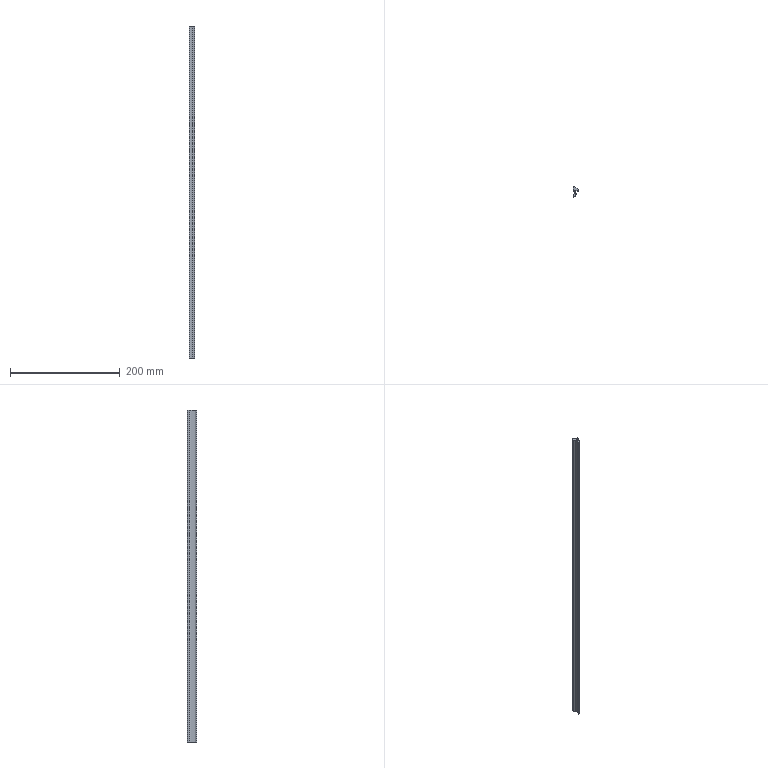Part | SolidWorks | features BaseBody 1, MoveFace 1 | 1 solid | 20 faces | box 10.8 x 17.5 x 606 mm | volume 47753 mm3 | cylinder 11 | plane 9 | commonest cylinder face diameters 1.6 x2 14 x2 0.4 x1 0.6 x1 0.8 x1 2.6 x1
STEP:
#1=CARTESIAN_POINT('',(-3.236,-11.055,506.));
#2=VERTEX_POINT('',#1);
#3=CARTESIAN_POINT('',(-4.3,-10.3,506.));
#4=VERTEX_POINT('',#3);
#5=CARTESIAN_POINT('',(-3.5,-10.3,506.));
#6=DIRECTION('',(0.,0.,-1.));
#7=DIRECTION('',(1.,0.,0.));
#8=AXIS2_PLACEMENT_3D('',#5,#6,#7);
#9=CIRCLE('',#8,0.8);
#10=EDGE_CURVE('',#2,#4,#9,.T.);
#11=ORIENTED_EDGE('',*,*,#10,.T.);
#12=CARTESIAN_POINT('',(-4.3,-10.3,-100.));
#13=VERTEX_POINT('',#12);
#14=CARTESIAN_POINT('',(-4.3,-10.3,-100.));
#15=DIRECTION('',(0.,0.,-1.));
#16=VECTOR('',#15,1000.);
#17=LINE('',#14,#16);
#18=EDGE_CURVE('',#4,#13,#17,.T.);
#19=ORIENTED_EDGE('',*,*,#18,.T.);
#20=CARTESIAN_POINT('',(-3.236,-11.055,-100.));
#21=VERTEX_POINT('',#20);
#22=CARTESIAN_POINT('',(-3.5,-10.3,-100.));
#23=DIRECTION('',(0.,0.,1.));
#24=DIRECTION('',(-1.,0.,0.));
#25=AXIS2_PLACEMENT_3D('',#22,#23,#24);
#26=CIRCLE('',#25,0.8);
#27=EDGE_CURVE('',#13,#21,#26,.T.);
#28=ORIENTED_EDGE('',*,*,#27,.T.);
#29=CARTESIAN_POINT('',(-3.236,-11.055,-100.));
#30=DIRECTION('',(0.,0.,-1.));
#31=VECTOR('',#30,1000.);
#32=LINE('',#29,#31);
#33=EDGE_CURVE('',#2,#21,#32,.T.);
#34=ORIENTED_EDGE('',*,*,#33,.F.);
#35=EDGE_LOOP('',(#11,#19,#28,#34));
#36=FACE_OUTER_BOUND('',#35,.T.);
#37=CARTESIAN_POINT('',(-3.5,-10.3,-100.));
#38=DIRECTION('',(0.,0.,-1.));
#39=DIRECTION('',(-1.,0.,0.));
#40=AXIS2_PLACEMENT_3D('',#37,#38,#39);
#41=CYLINDRICAL_SURFACE('',#40,0.8);
#42=ADVANCED_FACE('',(#36),#41,.T.);
#43=CARTESIAN_POINT('',(1.184,-6.397,-100.));
#44=VERTEX_POINT('',#43);
#45=CARTESIAN_POINT('',(-5.702,-4.29,-100.));
#46=DIRECTION('',(0.,0.,1.));
#47=DIRECTION('',(-1.,0.,0.));
#48=AXIS2_PLACEMENT_3D('',#45,#46,#47);
#49=CIRCLE('',#48,7.201);
#50=EDGE_CURVE('',#21,#44,#49,.T.);
#51=ORIENTED_EDGE('',*,*,#50,.T.);
#52=CARTESIAN_POINT('',(1.184,-6.397,506.));
#53=VERTEX_POINT('',#52);
#54=CARTESIAN_POINT('',(1.184,-6.397,-100.));
#55=DIRECTION('',(0.,0.,1.));
#56=VECTOR('',#55,1000.);
#57=LINE('',#54,#56);
#58=EDGE_CURVE('',#44,#53,#57,.T.);
#59=ORIENTED_EDGE('',*,*,#58,.T.);
#60=CARTESIAN_POINT('',(-5.702,-4.29,506.));
#61=DIRECTION('',(0.,0.,-1.));
#62=DIRECTION('',(1.,0.,0.));
#63=AXIS2_PLACEMENT_3D('',#60,#61,#62);
#64=CIRCLE('',#63,7.201);
#65=EDGE_CURVE('',#53,#2,#64,.T.);
#66=ORIENTED_EDGE('',*,*,#65,.T.);
#67=ORIENTED_EDGE('',*,*,#33,.T.);
#68=EDGE_LOOP('',(#51,#59,#66,#67));
#69=FACE_OUTER_BOUND('',#68,.T.);
#70=CARTESIAN_POINT('',(-5.702,-4.29,-100.));
#71=DIRECTION('',(0.,0.,-1.));
#72=DIRECTION('',(-1.,0.,0.));
#73=AXIS2_PLACEMENT_3D('',#70,#71,#72);
#74=CYLINDRICAL_SURFACE('',#73,7.201);
#75=ADVANCED_FACE('',(#69),#74,.T.);
#76=CARTESIAN_POINT('',(0.9,-6.,-100.));
#77=VERTEX_POINT('',#76);
#78=CARTESIAN_POINT('',(0.9,-6.3,-100.));
#79=DIRECTION('',(0.,0.,1.));
#80=DIRECTION('',(-1.,0.,0.));
#81=AXIS2_PLACEMENT_3D('',#78,#79,#80);
#82=CIRCLE('',#81,0.3);
#83=EDGE_CURVE('',#44,#77,#82,.T.);
#84=ORIENTED_EDGE('',*,*,#83,.T.);
#85=CARTESIAN_POINT('',(0.9,-6.,506.));
#86=VERTEX_POINT('',#85);
#87=CARTESIAN_POINT('',(0.9,-6.,-100.));
#88=DIRECTION('',(0.,0.,1.));
#89=VECTOR('',#88,1000.);
#90=LINE('',#87,#89);
#91=EDGE_CURVE('',#77,#86,#90,.T.);
#92=ORIENTED_EDGE('',*,*,#91,.T.);
#93=CARTESIAN_POINT('',(0.9,-6.3,506.));
#94=DIRECTION('',(0.,0.,-1.));
#95=DIRECTION('',(1.,0.,0.));
#96=AXIS2_PLACEMENT_3D('',#93,#94,#95);
#97=CIRCLE('',#96,0.3);
#98=EDGE_CURVE('',#86,#53,#97,.T.);
#99=ORIENTED_EDGE('',*,*,#98,.T.);
#100=ORIENTED_EDGE('',*,*,#58,.F.);
#101=EDGE_LOOP('',(#84,#92,#99,#100));
#102=FACE_OUTER_BOUND('',#101,.T.);
#103=CARTESIAN_POINT('',(0.9,-6.3,-100.));
#104=DIRECTION('',(0.,0.,-1.));
#105=DIRECTION('',(-1.,0.,0.));
#106=AXIS2_PLACEMENT_3D('',#103,#104,#105);
#107=CYLINDRICAL_SURFACE('',#106,0.3);
#108=ADVANCED_FACE('',(#102),#107,.T.);
#109=CARTESIAN_POINT('',(-2.5,-0.5,-100.));
#110=VERTEX_POINT('',#109);
#111=CARTESIAN_POINT('',(-2.5,-6.153,-100.));
#112=VERTEX_POINT('',#111);
#113=CARTESIAN_POINT('',(-2.5,-6.397,-100.));
#114=DIRECTION('',(0.,-1.,0.));
#115=VECTOR('',#114,1000.);
#116=LINE('',#113,#115);
#117=EDGE_CURVE('',#110,#112,#116,.T.);
#118=ORIENTED_EDGE('',*,*,#117,.F.);
#119=CARTESIAN_POINT('',(-4.2,1.695,-100.));
#120=VERTEX_POINT('',#119);
#121=CARTESIAN_POINT('',(-1.701,1.875,-100.));
#122=DIRECTION('',(0.,0.,1.));
#123=DIRECTION('',(-1.,0.,0.));
#124=AXIS2_PLACEMENT_3D('',#121,#122,#123);
#125=CIRCLE('',#124,2.506);
#126=EDGE_CURVE('',#120,#110,#125,.T.);
#127=ORIENTED_EDGE('',*,*,#126,.F.);
#128=CARTESIAN_POINT('',(-4.2,5.1,-100.));
#129=VERTEX_POINT('',#128);
#130=CARTESIAN_POINT('',(-4.2,-6.397,-100.));
#131=DIRECTION('',(0.,-1.,0.));
#132=VECTOR('',#131,1000.);
#133=LINE('',#130,#132);
#134=EDGE_CURVE('',#129,#120,#133,.T.);
#135=ORIENTED_EDGE('',*,*,#134,.F.);
#136=CARTESIAN_POINT('',(-2.892,6.4,-100.));
#137=VERTEX_POINT('',#136);
#138=CARTESIAN_POINT('',(-2.9,5.1,-100.));
#139=DIRECTION('',(0.,0.,1.));
#140=DIRECTION('',(-1.,0.,0.));
#141=AXIS2_PLACEMENT_3D('',#138,#139,#140);
#142=CIRCLE('',#141,1.3);
#143=EDGE_CURVE('',#137,#129,#142,.T.);
#144=ORIENTED_EDGE('',*,*,#143,.F.);
#145=CARTESIAN_POINT('',(0.5,5.5,-100.));
#146=VERTEX_POINT('',#145);
#147=CARTESIAN_POINT('',(-2.934,-0.5999,-100.));
#148=DIRECTION('',(0.,0.,1.));
#149=DIRECTION('',(-1.,0.,0.));
#150=AXIS2_PLACEMENT_3D('',#147,#148,#149);
#151=CIRCLE('',#150,7.);
#152=EDGE_CURVE('',#146,#137,#151,.T.);
#153=ORIENTED_EDGE('',*,*,#152,.F.);
#154=CARTESIAN_POINT('',(5.5,1.7,-100.));
#155=VERTEX_POINT('',#154);
#156=CARTESIAN_POINT('',(5.5,1.7,-100.));
#157=DIRECTION('',(-0.7962,0.6051,0.));
#158=VECTOR('',#157,1000.);
#159=LINE('',#156,#158);
#160=EDGE_CURVE('',#155,#146,#159,.T.);
#161=ORIENTED_EDGE('',*,*,#160,.F.);
#162=CARTESIAN_POINT('',(6.458,-0.2215,-100.));
#163=VERTEX_POINT('',#162);
#164=CARTESIAN_POINT('',(6.458,-0.2215,-100.));
#165=DIRECTION('',(-0.4462,0.8949,0.));
#166=VECTOR('',#165,1000.);
#167=LINE('',#164,#166);
#168=EDGE_CURVE('',#163,#155,#167,.T.);
#169=ORIENTED_EDGE('',*,*,#168,.F.);
#170=CARTESIAN_POINT('',(5.895,-0.7433,-100.));
#171=VERTEX_POINT('',#170);
#172=CARTESIAN_POINT('',(6.1,-0.4,-100.));
#173=DIRECTION('',(0.,0.,1.));
#174=DIRECTION('',(-1.,0.,0.));
#175=AXIS2_PLACEMENT_3D('',#172,#173,#174);
#176=CIRCLE('',#175,0.4);
#177=EDGE_CURVE('',#171,#163,#176,.T.);
#178=ORIENTED_EDGE('',*,*,#177,.F.);
#179=CARTESIAN_POINT('',(3.,0.,-100.));
#180=VERTEX_POINT('',#179);
#181=CARTESIAN_POINT('',(2.746,-6.995,-100.));
#182=DIRECTION('',(0.,0.,-1.));
#183=DIRECTION('',(-1.,0.,0.));
#184=AXIS2_PLACEMENT_3D('',#181,#182,#183);
#185=CIRCLE('',#184,7.);
#186=EDGE_CURVE('',#180,#171,#185,.T.);
#187=ORIENTED_EDGE('',*,*,#186,.F.);
#188=CARTESIAN_POINT('',(0.,0.,-100.));
#189=VERTEX_POINT('',#188);
#190=CARTESIAN_POINT('',(-6.814,0.,-100.));
#191=DIRECTION('',(1.,0.,0.));
#192=VECTOR('',#191,1000.);
#193=LINE('',#190,#192);
#194=EDGE_CURVE('',#189,#180,#193,.T.);
#195=ORIENTED_EDGE('',*,*,#194,.F.);
#196=CARTESIAN_POINT('',(0.,-5.8,-100.));
#197=VERTEX_POINT('',#196);
#198=CARTESIAN_POINT('',(0.,-6.397,-100.));
#199=DIRECTION('',(0.,1.,0.));
#200=VECTOR('',#199,1000.);
#201=LINE('',#198,#200);
#202=EDGE_CURVE('',#197,#189,#201,.T.);
#203=ORIENTED_EDGE('',*,*,#202,.F.);
#204=CARTESIAN_POINT('',(0.2,-6.,-100.));
#205=VERTEX_POINT('',#204);
#206=CARTESIAN_POINT('',(0.2,-5.8,-100.));
#207=DIRECTION('',(0.,0.,1.));
#208=DIRECTION('',(-1.,0.,0.));
#209=AXIS2_PLACEMENT_3D('',#206,#207,#208);
#210=CIRCLE('',#209,0.2);
#211=EDGE_CURVE('',#197,#205,#210,.T.);
#212=ORIENTED_EDGE('',*,*,#211,.T.);
#213=CARTESIAN_POINT('',(-6.814,-6.,-100.));
#214=DIRECTION('',(-1.,0.,0.));
#215=VECTOR('',#214,1000.);
#216=LINE('',#213,#215);
#217=EDGE_CURVE('',#77,#205,#216,.T.);
#218=ORIENTED_EDGE('',*,*,#217,.F.);
#219=ORIENTED_EDGE('',*,*,#83,.F.);
#220=ORIENTED_EDGE('',*,*,#50,.F.);
#221=ORIENTED_EDGE('',*,*,#27,.F.);
#222=CARTESIAN_POINT('',(-3.998,-9.674,-100.));
#223=VERTEX_POINT('',#222);
#224=CARTESIAN_POINT('',(-3.5,-10.3,-100.));
#225=DIRECTION('',(0.,0.,1.));
#226=DIRECTION('',(-1.,0.,0.));
#227=AXIS2_PLACEMENT_3D('',#224,#225,#226);
#228=CIRCLE('',#227,0.8);
#229=EDGE_CURVE('',#223,#13,#228,.T.);
#230=ORIENTED_EDGE('',*,*,#229,.F.);
#231=CARTESIAN_POINT('',(-6.814,-6.397,-100.));
#232=DIRECTION('',(0.,0.,-1.));
#233=DIRECTION('',(-1.,0.,0.));
#234=AXIS2_PLACEMENT_3D('',#231,#232,#233);
#235=CIRCLE('',#234,4.321);
#236=EDGE_CURVE('',#112,#223,#235,.T.);
#237=ORIENTED_EDGE('',*,*,#236,.F.);
#238=EDGE_LOOP('',(#118,#127,#135,#144,#153,#161,#169,#178,#187,#195,#203,#212,#218,#219,#220,#221,#230,#237));
#239=FACE_OUTER_BOUND('',#238,.T.);
#240=CARTESIAN_POINT('',(-6.814,-6.397,-100.));
#241=DIRECTION('',(0.,0.,1.));
#242=DIRECTION('',(1.,0.,0.));
#243=AXIS2_PLACEMENT_3D('',#240,#241,#242);
#244=PLANE('',#243);
#245=ADVANCED_FACE('',(#239),#244,.F.);
#246=ORIENTED_EDGE('',*,*,#18,.F.);
#247=CARTESIAN_POINT('',(-3.998,-9.674,506.));
#248=VERTEX_POINT('',#247);
#249=CARTESIAN_POINT('',(-3.5,-10.3,506.));
#250=DIRECTION('',(0.,0.,-1.));
#251=DIRECTION('',(1.,0.,0.));
#252=AXIS2_PLACEMENT_3D('',#249,#250,#251);
#253=CIRCLE('',#252,0.8);
#254=EDGE_CURVE('',#4,#248,#253,.T.);
#255=ORIENTED_EDGE('',*,*,#254,.T.);
#256=CARTESIAN_POINT('',(-3.998,-9.674,-100.));
#257=DIRECTION('',(0.,0.,-1.));
#258=VECTOR('',#257,1000.);
#259=LINE('',#256,#258);
#260=EDGE_CURVE('',#248,#223,#259,.T.);
#261=ORIENTED_EDGE('',*,*,#260,.T.);
#262=ORIENTED_EDGE('',*,*,#229,.T.);
#263=EDGE_LOOP('',(#246,#255,#261,#262));
#264=FACE_OUTER_BOUND('',#263,.T.);
#265=CARTESIAN_POINT('',(-3.5,-10.3,-100.));
#266=DIRECTION('',(0.,0.,-1.));
#267=DIRECTION('',(-1.,0.,0.));
#268=AXIS2_PLACEMENT_3D('',#265,#266,#267);
#269=CYLINDRICAL_SURFACE('',#268,0.8);
#270=ADVANCED_FACE('',(#264),#269,.T.);
#271=CARTESIAN_POINT('',(-4.2,1.695,506.));
#272=VERTEX_POINT('',#271);
#273=CARTESIAN_POINT('',(-2.5,-0.5,506.));
#274=VERTEX_POINT('',#273);
#275=CARTESIAN_POINT('',(-1.701,1.875,506.));
#276=DIRECTION('',(0.,0.,1.));
#277=DIRECTION('',(1.,0.,0.));
#278=AXIS2_PLACEMENT_3D('',#275,#276,#277);
#279=CIRCLE('',#278,2.506);
#280=EDGE_CURVE('',#272,#274,#279,.T.);
#281=ORIENTED_EDGE('',*,*,#280,.T.);
#282=CARTESIAN_POINT('',(-2.5,-6.153,506.));
#283=VERTEX_POINT('',#282);
#284=CARTESIAN_POINT('',(-2.5,-6.397,506.));
#285=DIRECTION('',(0.,-1.,0.));
#286=VECTOR('',#285,1000.);
#287=LINE('',#284,#286);
#288=EDGE_CURVE('',#274,#283,#287,.T.);
#289=ORIENTED_EDGE('',*,*,#288,.T.);
#290=CARTESIAN_POINT('',(-6.814,-6.397,506.));
#291=DIRECTION('',(0.,0.,-1.));
#292=DIRECTION('',(1.,0.,0.));
#293=AXIS2_PLACEMENT_3D('',#290,#291,#292);
#294=CIRCLE('',#293,4.321);
#295=EDGE_CURVE('',#283,#248,#294,.T.);
#296=ORIENTED_EDGE('',*,*,#295,.T.);
#297=ORIENTED_EDGE('',*,*,#254,.F.);
#298=ORIENTED_EDGE('',*,*,#10,.F.);
#299=ORIENTED_EDGE('',*,*,#65,.F.);
#300=ORIENTED_EDGE('',*,*,#98,.F.);
#301=CARTESIAN_POINT('',(0.2,-6.,506.));
#302=VERTEX_POINT('',#301);
#303=CARTESIAN_POINT('',(-6.814,-6.,506.));
#304=DIRECTION('',(-1.,0.,0.));
#305=VECTOR('',#304,1000.);
#306=LINE('',#303,#305);
#307=EDGE_CURVE('',#86,#302,#306,.T.);
#308=ORIENTED_EDGE('',*,*,#307,.T.);
#309=CARTESIAN_POINT('',(0.,-5.8,506.));
#310=VERTEX_POINT('',#309);
#311=CARTESIAN_POINT('',(0.2,-5.8,506.));
#312=DIRECTION('',(0.,0.,-1.));
#313=DIRECTION('',(1.,0.,0.));
#314=AXIS2_PLACEMENT_3D('',#311,#312,#313);
#315=CIRCLE('',#314,0.2);
#316=EDGE_CURVE('',#302,#310,#315,.T.);
#317=ORIENTED_EDGE('',*,*,#316,.T.);
#318=CARTESIAN_POINT('',(0.,0.,506.));
#319=VERTEX_POINT('',#318);
#320=CARTESIAN_POINT('',(0.,-6.397,506.));
#321=DIRECTION('',(0.,1.,0.));
#322=VECTOR('',#321,1000.);
#323=LINE('',#320,#322);
#324=EDGE_CURVE('',#310,#319,#323,.T.);
#325=ORIENTED_EDGE('',*,*,#324,.T.);
#326=CARTESIAN_POINT('',(3.,0.,506.));
#327=VERTEX_POINT('',#326);
#328=CARTESIAN_POINT('',(-6.814,0.,506.));
#329=DIRECTION('',(1.,0.,0.));
#330=VECTOR('',#329,1000.);
#331=LINE('',#328,#330);
#332=EDGE_CURVE('',#319,#327,#331,.T.);
#333=ORIENTED_EDGE('',*,*,#332,.T.);
#334=CARTESIAN_POINT('',(5.895,-0.7433,506.));
#335=VERTEX_POINT('',#334);
#336=CARTESIAN_POINT('',(2.746,-6.995,506.));
#337=DIRECTION('',(0.,0.,-1.));
#338=DIRECTION('',(1.,0.,0.));
#339=AXIS2_PLACEMENT_3D('',#336,#337,#338);
#340=CIRCLE('',#339,7.);
#341=EDGE_CURVE('',#327,#335,#340,.T.);
#342=ORIENTED_EDGE('',*,*,#341,.T.);
#343=CARTESIAN_POINT('',(6.458,-0.2215,506.));
#344=VERTEX_POINT('',#343);
#345=CARTESIAN_POINT('',(6.1,-0.4,506.));
#346=DIRECTION('',(0.,0.,-1.));
#347=DIRECTION('',(1.,0.,0.));
#348=AXIS2_PLACEMENT_3D('',#345,#346,#347);
#349=CIRCLE('',#348,0.4);
#350=EDGE_CURVE('',#344,#335,#349,.T.);
#351=ORIENTED_EDGE('',*,*,#350,.F.);
#352=CARTESIAN_POINT('',(5.5,1.7,506.));
#353=VERTEX_POINT('',#352);
#354=CARTESIAN_POINT('',(6.282,0.1323,506.));
#355=DIRECTION('',(-0.4462,0.8949,0.));
#356=VECTOR('',#355,1000.);
#357=LINE('',#354,#356);
#358=EDGE_CURVE('',#344,#353,#357,.T.);
#359=ORIENTED_EDGE('',*,*,#358,.T.);
#360=CARTESIAN_POINT('',(0.5,5.5,506.));
#361=VERTEX_POINT('',#360);
#362=CARTESIAN_POINT('',(1.595,4.668,506.));
#363=DIRECTION('',(-0.7962,0.6051,0.));
#364=VECTOR('',#363,1000.);
#365=LINE('',#362,#364);
#366=EDGE_CURVE('',#353,#361,#365,.T.);
#367=ORIENTED_EDGE('',*,*,#366,.T.);
#368=CARTESIAN_POINT('',(-2.892,6.4,506.));
#369=VERTEX_POINT('',#368);
#370=CARTESIAN_POINT('',(-2.934,-0.5999,506.));
#371=DIRECTION('',(0.,0.,1.));
#372=DIRECTION('',(1.,0.,0.));
#373=AXIS2_PLACEMENT_3D('',#370,#371,#372);
#374=CIRCLE('',#373,7.);
#375=EDGE_CURVE('',#361,#369,#374,.T.);
#376=ORIENTED_EDGE('',*,*,#375,.T.);
#377=CARTESIAN_POINT('',(-4.2,5.1,506.));
#378=VERTEX_POINT('',#377);
#379=CARTESIAN_POINT('',(-2.9,5.1,506.));
#380=DIRECTION('',(0.,0.,1.));
#381=DIRECTION('',(1.,0.,0.));
#382=AXIS2_PLACEMENT_3D('',#379,#380,#381);
#383=CIRCLE('',#382,1.3);
#384=EDGE_CURVE('',#369,#378,#383,.T.);
#385=ORIENTED_EDGE('',*,*,#384,.T.);
#386=CARTESIAN_POINT('',(-4.2,-6.397,506.));
#387=DIRECTION('',(0.,-1.,0.));
#388=VECTOR('',#387,1000.);
#389=LINE('',#386,#388);
#390=EDGE_CURVE('',#378,#272,#389,.T.);
#391=ORIENTED_EDGE('',*,*,#390,.T.);
#392=EDGE_LOOP('',(#281,#289,#296,#297,#298,#299,#300,#308,#317,#325,#333,#342,#351,#359,#367,#376,#385,#391));
#393=FACE_OUTER_BOUND('',#392,.T.);
#394=CARTESIAN_POINT('',(-6.814,-6.397,506.));
#395=DIRECTION('',(0.,0.,1.));
#396=DIRECTION('',(1.,0.,0.));
#397=AXIS2_PLACEMENT_3D('',#394,#395,#396);
#398=PLANE('',#397);
#399=ADVANCED_FACE('',(#393),#398,.T.);
#400=ORIENTED_EDGE('',*,*,#217,.T.);
#401=CARTESIAN_POINT('',(0.2,-6.,-100.));
#402=DIRECTION('',(0.,0.,1.));
#403=VECTOR('',#402,1000.);
#404=LINE('',#401,#403);
#405=EDGE_CURVE('',#205,#302,#404,.T.);
#406=ORIENTED_EDGE('',*,*,#405,.T.);
#407=ORIENTED_EDGE('',*,*,#307,.F.);
#408=ORIENTED_EDGE('',*,*,#91,.F.);
#409=EDGE_LOOP('',(#400,#406,#407,#408));
#410=FACE_OUTER_BOUND('',#409,.T.);
#411=CARTESIAN_POINT('',(0.9,-6.,-100.));
#412=DIRECTION('',(0.,1.,0.));
#413=DIRECTION('',(0.,0.,1.));
#414=AXIS2_PLACEMENT_3D('',#411,#412,#413);
#415=PLANE('',#414);
#416=ADVANCED_FACE('',(#410),#415,.T.);
#417=CARTESIAN_POINT('',(-2.5,-6.153,-100.));
#418=DIRECTION('',(0.,0.,1.));
#419=VECTOR('',#418,1000.);
#420=LINE('',#417,#419);
#421=EDGE_CURVE('',#112,#283,#420,.T.);
#422=ORIENTED_EDGE('',*,*,#421,.F.);
#423=ORIENTED_EDGE('',*,*,#236,.T.);
#424=ORIENTED_EDGE('',*,*,#260,.F.);
#425=ORIENTED_EDGE('',*,*,#295,.F.);
#426=EDGE_LOOP('',(#422,#423,#424,#425));
#427=FACE_OUTER_BOUND('',#426,.T.);
#428=CARTESIAN_POINT('',(-6.814,-6.397,-100.));
#429=DIRECTION('',(0.,0.,-1.));
#430=DIRECTION('',(-1.,0.,0.));
#431=AXIS2_PLACEMENT_3D('',#428,#429,#430);
#432=CYLINDRICAL_SURFACE('',#431,4.321);
#433=ADVANCED_FACE('',(#427),#432,.F.);
#434=ORIENTED_EDGE('',*,*,#117,.T.);
#435=ORIENTED_EDGE('',*,*,#421,.T.);
#436=ORIENTED_EDGE('',*,*,#288,.F.);
#437=CARTESIAN_POINT('',(-2.5,-0.5,-100.));
#438=DIRECTION('',(0.,0.,-1.));
#439=VECTOR('',#438,1000.);
#440=LINE('',#437,#439);
#441=EDGE_CURVE('',#274,#110,#440,.T.);
#442=ORIENTED_EDGE('',*,*,#441,.T.);
#443=EDGE_LOOP('',(#434,#435,#436,#442));
#444=FACE_OUTER_BOUND('',#443,.T.);
#445=CARTESIAN_POINT('',(-2.5,-0.5,-100.));
#446=DIRECTION('',(-1.,0.,0.));
#447=DIRECTION('',(0.,0.,1.));
#448=AXIS2_PLACEMENT_3D('',#445,#446,#447);
#449=PLANE('',#448);
#450=ADVANCED_FACE('',(#444),#449,.T.);
#451=ORIENTED_EDGE('',*,*,#126,.T.);
#452=ORIENTED_EDGE('',*,*,#441,.F.);
#453=ORIENTED_EDGE('',*,*,#280,.F.);
#454=CARTESIAN_POINT('',(-4.2,1.695,-100.));
#455=DIRECTION('',(0.,0.,-1.));
#456=VECTOR('',#455,1000.);
#457=LINE('',#454,#456);
#458=EDGE_CURVE('',#272,#120,#457,.T.);
#459=ORIENTED_EDGE('',*,*,#458,.T.);
#460=EDGE_LOOP('',(#451,#452,#453,#459));
#461=FACE_OUTER_BOUND('',#460,.T.);
#462=CARTESIAN_POINT('',(-1.701,1.875,-100.));
#463=DIRECTION('',(0.,0.,-1.));
#464=DIRECTION('',(-1.,0.,0.));
#465=AXIS2_PLACEMENT_3D('',#462,#463,#464);
#466=CYLINDRICAL_SURFACE('',#465,2.506);
#467=ADVANCED_FACE('',(#461),#466,.T.);
#468=ORIENTED_EDGE('',*,*,#134,.T.);
#469=ORIENTED_EDGE('',*,*,#458,.F.);
#470=ORIENTED_EDGE('',*,*,#390,.F.);
#471=CARTESIAN_POINT('',(-4.2,5.1,-100.));
#472=DIRECTION('',(0.,0.,-1.));
#473=VECTOR('',#472,1000.);
#474=LINE('',#471,#473);
#475=EDGE_CURVE('',#378,#129,#474,.T.);
#476=ORIENTED_EDGE('',*,*,#475,.T.);
#477=EDGE_LOOP('',(#468,#469,#470,#476));
#478=FACE_OUTER_BOUND('',#477,.T.);
#479=CARTESIAN_POINT('',(-4.2,5.1,-100.));
#480=DIRECTION('',(-1.,0.,0.));
#481=DIRECTION('',(0.,0.,1.));
#482=AXIS2_PLACEMENT_3D('',#479,#480,#481);
#483=PLANE('',#482);
#484=ADVANCED_FACE('',(#478),#483,.T.);
#485=ORIENTED_EDGE('',*,*,#143,.T.);
#486=ORIENTED_EDGE('',*,*,#475,.F.);
#487=ORIENTED_EDGE('',*,*,#384,.F.);
#488=CARTESIAN_POINT('',(-2.892,6.4,-100.));
#489=DIRECTION('',(0.,0.,-1.));
#490=VECTOR('',#489,1000.);
#491=LINE('',#488,#490);
#492=EDGE_CURVE('',#369,#137,#491,.T.);
#493=ORIENTED_EDGE('',*,*,#492,.T.);
#494=EDGE_LOOP('',(#485,#486,#487,#493));
#495=FACE_OUTER_BOUND('',#494,.T.);
#496=CARTESIAN_POINT('',(-2.9,5.1,-100.));
#497=DIRECTION('',(0.,0.,-1.));
#498=DIRECTION('',(-1.,0.,0.));
#499=AXIS2_PLACEMENT_3D('',#496,#497,#498);
#500=CYLINDRICAL_SURFACE('',#499,1.3);
#501=ADVANCED_FACE('',(#495),#500,.T.);
#502=ORIENTED_EDGE('',*,*,#152,.T.);
#503=ORIENTED_EDGE('',*,*,#492,.F.);
#504=ORIENTED_EDGE('',*,*,#375,.F.);
#505=CARTESIAN_POINT('',(0.5,5.5,-100.));
#506=DIRECTION('',(0.,0.,-1.));
#507=VECTOR('',#506,1000.);
#508=LINE('',#505,#507);
#509=EDGE_CURVE('',#361,#146,#508,.T.);
#510=ORIENTED_EDGE('',*,*,#509,.T.);
#511=EDGE_LOOP('',(#502,#503,#504,#510));
#512=FACE_OUTER_BOUND('',#511,.T.);
#513=CARTESIAN_POINT('',(-2.934,-0.5999,-100.));
#514=DIRECTION('',(0.,0.,-1.));
#515=DIRECTION('',(-1.,0.,0.));
#516=AXIS2_PLACEMENT_3D('',#513,#514,#515);
#517=CYLINDRICAL_SURFACE('',#516,7.);
#518=ADVANCED_FACE('',(#512),#517,.T.);
#519=ORIENTED_EDGE('',*,*,#160,.T.);
#520=ORIENTED_EDGE('',*,*,#509,.F.);
#521=ORIENTED_EDGE('',*,*,#366,.F.);
#522=CARTESIAN_POINT('',(5.5,1.7,-100.));
#523=DIRECTION('',(0.,0.,-1.));
#524=VECTOR('',#523,1000.);
#525=LINE('',#522,#524);
#526=EDGE_CURVE('',#353,#155,#525,.T.);
#527=ORIENTED_EDGE('',*,*,#526,.T.);
#528=EDGE_LOOP('',(#519,#520,#521,#527));
#529=FACE_OUTER_BOUND('',#528,.T.);
#530=CARTESIAN_POINT('',(5.5,1.7,-100.));
#531=DIRECTION('',(0.6051,0.7962,0.));
#532=DIRECTION('',(-0.7962,0.6051,0.));
#533=AXIS2_PLACEMENT_3D('',#530,#531,#532);
#534=PLANE('',#533);
#535=ADVANCED_FACE('',(#529),#534,.T.);
#536=ORIENTED_EDGE('',*,*,#168,.T.);
#537=ORIENTED_EDGE('',*,*,#526,.F.);
#538=ORIENTED_EDGE('',*,*,#358,.F.);
#539=CARTESIAN_POINT('',(6.458,-0.2215,-100.));
#540=DIRECTION('',(0.,0.,-1.));
#541=VECTOR('',#540,1000.);
#542=LINE('',#539,#541);
#543=EDGE_CURVE('',#344,#163,#542,.T.);
#544=ORIENTED_EDGE('',*,*,#543,.T.);
#545=EDGE_LOOP('',(#536,#537,#538,#544));
#546=FACE_OUTER_BOUND('',#545,.T.);
#547=CARTESIAN_POINT('',(6.458,-0.2215,-100.));
#548=DIRECTION('',(0.8949,0.4462,0.));
#549=DIRECTION('',(-0.4462,0.8949,0.));
#550=AXIS2_PLACEMENT_3D('',#547,#548,#549);
#551=PLANE('',#550);
#552=ADVANCED_FACE('',(#546),#551,.T.);
#553=CARTESIAN_POINT('',(3.,0.,-100.));
#554=DIRECTION('',(0.,0.,1.));
#555=VECTOR('',#554,1000.);
#556=LINE('',#553,#555);
#557=EDGE_CURVE('',#180,#327,#556,.T.);
#558=ORIENTED_EDGE('',*,*,#557,.F.);
#559=ORIENTED_EDGE('',*,*,#186,.T.);
#560=CARTESIAN_POINT('',(5.895,-0.7433,-100.));
#561=DIRECTION('',(0.,0.,-1.));
#562=VECTOR('',#561,1000.);
#563=LINE('',#560,#562);
#564=EDGE_CURVE('',#335,#171,#563,.T.);
#565=ORIENTED_EDGE('',*,*,#564,.F.);
#566=ORIENTED_EDGE('',*,*,#341,.F.);
#567=EDGE_LOOP('',(#558,#559,#565,#566));
#568=FACE_OUTER_BOUND('',#567,.T.);
#569=CARTESIAN_POINT('',(2.746,-6.995,-100.));
#570=DIRECTION('',(0.,0.,-1.));
#571=DIRECTION('',(-1.,0.,0.));
#572=AXIS2_PLACEMENT_3D('',#569,#570,#571);
#573=CYLINDRICAL_SURFACE('',#572,7.);
#574=ADVANCED_FACE('',(#568),#573,.F.);
#575=ORIENTED_EDGE('',*,*,#194,.T.);
#576=ORIENTED_EDGE('',*,*,#557,.T.);
#577=ORIENTED_EDGE('',*,*,#332,.F.);
#578=CARTESIAN_POINT('',(0.,0.,-100.));
#579=DIRECTION('',(0.,0.,-1.));
#580=VECTOR('',#579,1000.);
#581=LINE('',#578,#580);
#582=EDGE_CURVE('',#319,#189,#581,.T.);
#583=ORIENTED_EDGE('',*,*,#582,.T.);
#584=EDGE_LOOP('',(#575,#576,#577,#583));
#585=FACE_OUTER_BOUND('',#584,.T.);
#586=CARTESIAN_POINT('',(0.,0.,-100.));
#587=DIRECTION('',(0.,-1.,0.));
#588=DIRECTION('',(0.,0.,-1.));
#589=AXIS2_PLACEMENT_3D('',#586,#587,#588);
#590=PLANE('',#589);
#591=ADVANCED_FACE('',(#585),#590,.T.);
#592=ORIENTED_EDGE('',*,*,#202,.T.);
#593=ORIENTED_EDGE('',*,*,#582,.F.);
#594=ORIENTED_EDGE('',*,*,#324,.F.);
#595=CARTESIAN_POINT('',(0.,-5.8,-100.));
#596=DIRECTION('',(0.,0.,-1.));
#597=VECTOR('',#596,1000.);
#598=LINE('',#595,#597);
#599=EDGE_CURVE('',#310,#197,#598,.T.);
#600=ORIENTED_EDGE('',*,*,#599,.T.);
#601=EDGE_LOOP('',(#592,#593,#594,#600));
#602=FACE_OUTER_BOUND('',#601,.T.);
#603=CARTESIAN_POINT('',(0.,-5.8,-100.));
#604=DIRECTION('',(1.,0.,0.));
#605=DIRECTION('',(0.,0.,-1.));
#606=AXIS2_PLACEMENT_3D('',#603,#604,#605);
#607=PLANE('',#606);
#608=ADVANCED_FACE('',(#602),#607,.T.);
#609=ORIENTED_EDGE('',*,*,#405,.F.);
#610=ORIENTED_EDGE('',*,*,#211,.F.);
#611=ORIENTED_EDGE('',*,*,#599,.F.);
#612=ORIENTED_EDGE('',*,*,#316,.F.);
#613=EDGE_LOOP('',(#609,#610,#611,#612));
#614=FACE_OUTER_BOUND('',#613,.T.);
#615=CARTESIAN_POINT('',(0.2,-5.8,-100.));
#616=DIRECTION('',(0.,0.,-1.));
#617=DIRECTION('',(-1.,0.,0.));
#618=AXIS2_PLACEMENT_3D('',#615,#616,#617);
#619=CYLINDRICAL_SURFACE('',#618,0.2);
#620=ADVANCED_FACE('',(#614),#619,.F.);
#621=ORIENTED_EDGE('',*,*,#177,.T.);
#622=ORIENTED_EDGE('',*,*,#543,.F.);
#623=ORIENTED_EDGE('',*,*,#350,.T.);
#624=ORIENTED_EDGE('',*,*,#564,.T.);
#625=EDGE_LOOP('',(#621,#622,#623,#624));
#626=FACE_OUTER_BOUND('',#625,.T.);
#627=CARTESIAN_POINT('',(6.1,-0.4,-100.));
#628=DIRECTION('',(0.,0.,-1.));
#629=DIRECTION('',(-1.,0.,0.));
#630=AXIS2_PLACEMENT_3D('',#627,#628,#629);
#631=CYLINDRICAL_SURFACE('',#630,0.4);
#632=ADVANCED_FACE('',(#626),#631,.T.);
#633=CLOSED_SHELL('',(#42,#75,#108,#245,#270,#399,#416,#433,#450,#467,#484,#501,#518,#535,#552,#574,#591,#608,#620,#632));
#634=MANIFOLD_SOLID_BREP('',#633);
#635=CARTESIAN_POINT('',(0.,0.,0.));
#636=DIRECTION('',(0.,0.,1.));
#637=DIRECTION('',(1.,0.,0.));
#638=AXIS2_PLACEMENT_3D('',#635,#636,#637);
#639=(LENGTH_UNIT()NAMED_UNIT(*)SI_UNIT(.MILLI.,.METRE.));
#640=UNCERTAINTY_MEASURE_WITH_UNIT(LENGTH_MEASURE(0.00001),#639,'','');
#641=(NAMED_UNIT(*)PLANE_ANGLE_UNIT()SI_UNIT($,.RADIAN.));
#642=(NAMED_UNIT(*)SI_UNIT($,.STERADIAN.)SOLID_ANGLE_UNIT());
#643=(GEOMETRIC_REPRESENTATION_CONTEXT(3)GLOBAL_UNCERTAINTY_ASSIGNED_CONTEXT((#640))GLOBAL_UNIT_ASSIGNED_CONTEXT((#639,#641,#642))REPRESENTATION_CONTEXT('',''));
#644=ADVANCED_BREP_SHAPE_REPRESENTATION('',(#634,#638),#643);